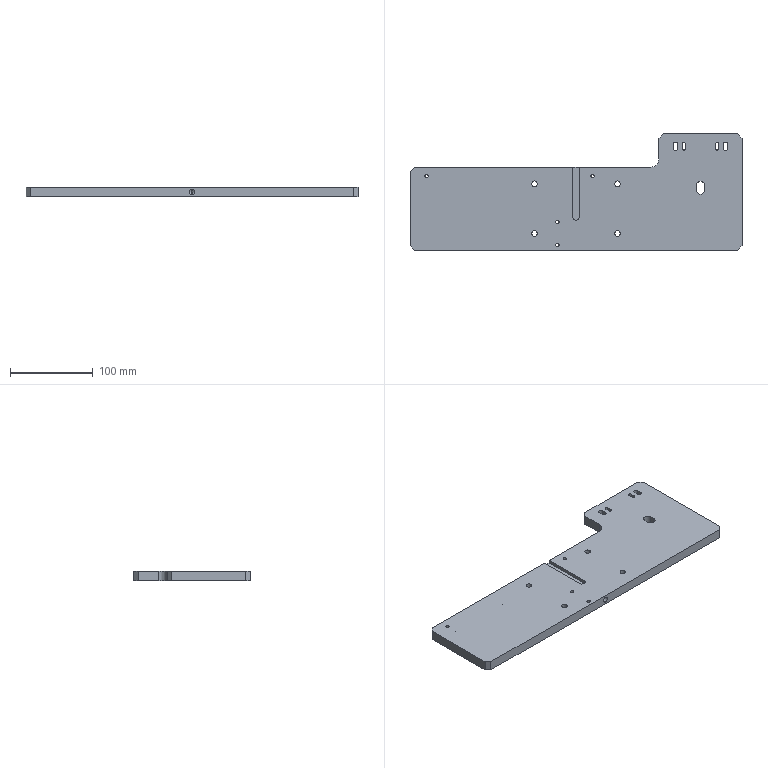Part | SolidWorks | features HoleWzd 5, ICE 5, Chamfer 1, Extrusion 1, Fillet 1 | 1 solid | 82 faces | box 400 x 140 x 12 mm | volume 518070 mm3 | cylinder 42 | plane 26 | cone 14 | commonest cylinder face diameters 3.3 x12 6.8 x10 4 x8 4.2 x4 5.5 x4 10.5 x2